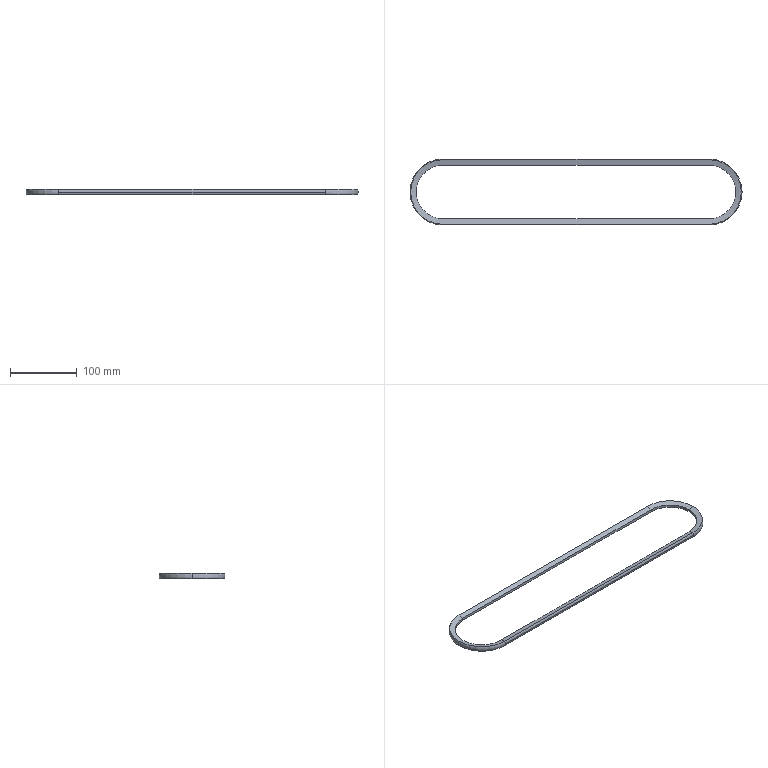Part | STEP file | BCC3 H16_10 | 1 solid | 24 faces | box 499.144 x 99.144 x 8 mm | volume 58375 mm3 | cylinder 8 | cone 6 | plane 6 | torus 4 | commonest cylinder face diameters 16 x4 81 x4